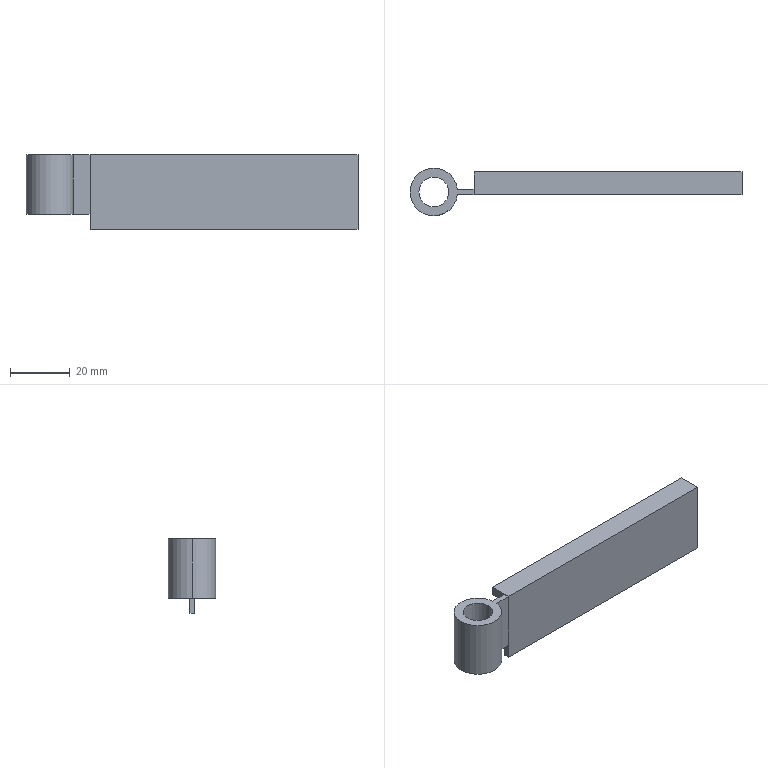Part | SolidWorks | features ICE 3, Extrusion 1 | 2 solids | 17 faces | box 111.5 x 16 x 25 mm | volume 8047 mm3 | plane 13 | cylinder 4 | commonest cylinder face diameters 10 x2 16 x2
STEP:
#1=CARTESIAN_POINT('',(-5.,0.,10.));
#2=VERTEX_POINT('',#1);
#3=CARTESIAN_POINT('',(5.,0.,10.));
#4=VERTEX_POINT('',#3);
#5=CARTESIAN_POINT('',(0.,0.,10.));
#6=DIRECTION('',(0.,0.,1.));
#7=DIRECTION('',(1.,0.,0.));
#8=AXIS2_PLACEMENT_3D('',#5,#6,#7);
#9=CIRCLE('',#8,5.);
#10=EDGE_CURVE('',#2,#4,#9,.T.);
#11=ORIENTED_EDGE('',*,*,#10,.T.);
#12=CARTESIAN_POINT('',(5.,0.,-10.));
#13=VERTEX_POINT('',#12);
#14=CARTESIAN_POINT('',(5.,0.,10.));
#15=DIRECTION('',(0.,0.,-1.));
#16=VECTOR('',#15,1000.);
#17=LINE('',#14,#16);
#18=EDGE_CURVE('',#4,#13,#17,.T.);
#19=ORIENTED_EDGE('',*,*,#18,.T.);
#20=CARTESIAN_POINT('',(-5.,0.,-10.));
#21=VERTEX_POINT('',#20);
#22=CARTESIAN_POINT('',(0.,0.,-10.));
#23=DIRECTION('',(0.,0.,1.));
#24=DIRECTION('',(1.,0.,0.));
#25=AXIS2_PLACEMENT_3D('',#22,#23,#24);
#26=CIRCLE('',#25,5.);
#27=EDGE_CURVE('',#21,#13,#26,.T.);
#28=ORIENTED_EDGE('',*,*,#27,.F.);
#29=CARTESIAN_POINT('',(-5.,0.,10.));
#30=DIRECTION('',(0.,0.,-1.));
#31=VECTOR('',#30,1000.);
#32=LINE('',#29,#31);
#33=EDGE_CURVE('',#2,#21,#32,.T.);
#34=ORIENTED_EDGE('',*,*,#33,.F.);
#35=EDGE_LOOP('',(#11,#19,#28,#34));
#36=FACE_OUTER_BOUND('',#35,.T.);
#37=CARTESIAN_POINT('',(0.,0.,10.));
#38=DIRECTION('',(0.,0.,-1.));
#39=DIRECTION('',(-1.,0.,0.));
#40=AXIS2_PLACEMENT_3D('',#37,#38,#39);
#41=CYLINDRICAL_SURFACE('',#40,5.);
#42=ADVANCED_FACE('',(#36),#41,.F.);
#43=CARTESIAN_POINT('',(-8.,0.,10.));
#44=VERTEX_POINT('',#43);
#45=CARTESIAN_POINT('',(7.945,-0.9375,10.));
#46=VERTEX_POINT('',#45);
#47=CARTESIAN_POINT('',(0.,0.,10.));
#48=DIRECTION('',(0.,0.,1.));
#49=DIRECTION('',(1.,0.,0.));
#50=AXIS2_PLACEMENT_3D('',#47,#48,#49);
#51=CIRCLE('',#50,8.);
#52=EDGE_CURVE('',#44,#46,#51,.T.);
#53=ORIENTED_EDGE('',*,*,#52,.F.);
#54=CARTESIAN_POINT('',(-8.,0.,-10.));
#55=VERTEX_POINT('',#54);
#56=CARTESIAN_POINT('',(-8.,0.,10.));
#57=DIRECTION('',(0.,0.,-1.));
#58=VECTOR('',#57,1000.);
#59=LINE('',#56,#58);
#60=EDGE_CURVE('',#44,#55,#59,.T.);
#61=ORIENTED_EDGE('',*,*,#60,.T.);
#62=CARTESIAN_POINT('',(7.945,-0.9375,-10.));
#63=VERTEX_POINT('',#62);
#64=CARTESIAN_POINT('',(0.,0.,-10.));
#65=DIRECTION('',(0.,0.,1.));
#66=DIRECTION('',(1.,0.,0.));
#67=AXIS2_PLACEMENT_3D('',#64,#65,#66);
#68=CIRCLE('',#67,8.);
#69=EDGE_CURVE('',#55,#63,#68,.T.);
#70=ORIENTED_EDGE('',*,*,#69,.T.);
#71=CARTESIAN_POINT('',(7.945,-0.9375,10.));
#72=DIRECTION('',(0.,0.,-1.));
#73=VECTOR('',#72,1000.);
#74=LINE('',#71,#73);
#75=EDGE_CURVE('',#46,#63,#74,.T.);
#76=ORIENTED_EDGE('',*,*,#75,.F.);
#77=EDGE_LOOP('',(#53,#61,#70,#76));
#78=FACE_OUTER_BOUND('',#77,.T.);
#79=CARTESIAN_POINT('',(0.,0.,10.));
#80=DIRECTION('',(0.,0.,-1.));
#81=DIRECTION('',(-1.,0.,0.));
#82=AXIS2_PLACEMENT_3D('',#79,#80,#81);
#83=CYLINDRICAL_SURFACE('',#82,8.);
#84=ADVANCED_FACE('',(#78),#83,.T.);
#85=ORIENTED_EDGE('',*,*,#60,.F.);
#86=CARTESIAN_POINT('',(7.945,0.9375,10.));
#87=VERTEX_POINT('',#86);
#88=CARTESIAN_POINT('',(0.,0.,10.));
#89=DIRECTION('',(0.,0.,1.));
#90=DIRECTION('',(1.,0.,0.));
#91=AXIS2_PLACEMENT_3D('',#88,#89,#90);
#92=CIRCLE('',#91,8.);
#93=EDGE_CURVE('',#87,#44,#92,.T.);
#94=ORIENTED_EDGE('',*,*,#93,.F.);
#95=CARTESIAN_POINT('',(7.945,0.9375,-10.));
#96=VERTEX_POINT('',#95);
#97=CARTESIAN_POINT('',(7.945,0.9375,10.));
#98=DIRECTION('',(0.,0.,1.));
#99=VECTOR('',#98,1000.);
#100=LINE('',#97,#99);
#101=EDGE_CURVE('',#96,#87,#100,.T.);
#102=ORIENTED_EDGE('',*,*,#101,.F.);
#103=CARTESIAN_POINT('',(0.,0.,-10.));
#104=DIRECTION('',(0.,0.,1.));
#105=DIRECTION('',(1.,0.,0.));
#106=AXIS2_PLACEMENT_3D('',#103,#104,#105);
#107=CIRCLE('',#106,8.);
#108=EDGE_CURVE('',#96,#55,#107,.T.);
#109=ORIENTED_EDGE('',*,*,#108,.T.);
#110=EDGE_LOOP('',(#85,#94,#102,#109));
#111=FACE_OUTER_BOUND('',#110,.T.);
#112=CARTESIAN_POINT('',(0.,0.,10.));
#113=DIRECTION('',(0.,0.,-1.));
#114=DIRECTION('',(-1.,0.,0.));
#115=AXIS2_PLACEMENT_3D('',#112,#113,#114);
#116=CYLINDRICAL_SURFACE('',#115,8.);
#117=ADVANCED_FACE('',(#111),#116,.T.);
#118=CARTESIAN_POINT('',(13.5,0.9375,10.));
#119=VERTEX_POINT('',#118);
#120=CARTESIAN_POINT('',(5.5,0.9375,10.));
#121=DIRECTION('',(-1.,0.,0.));
#122=VECTOR('',#121,1000.);
#123=LINE('',#120,#122);
#124=EDGE_CURVE('',#119,#87,#123,.T.);
#125=ORIENTED_EDGE('',*,*,#124,.T.);
#126=ORIENTED_EDGE('',*,*,#93,.T.);
#127=ORIENTED_EDGE('',*,*,#52,.T.);
#128=CARTESIAN_POINT('',(13.5,-0.9375,10.));
#129=VERTEX_POINT('',#128);
#130=CARTESIAN_POINT('',(5.5,-0.9375,10.));
#131=DIRECTION('',(1.,0.,0.));
#132=VECTOR('',#131,1000.);
#133=LINE('',#130,#132);
#134=EDGE_CURVE('',#46,#129,#133,.T.);
#135=ORIENTED_EDGE('',*,*,#134,.T.);
#136=CARTESIAN_POINT('',(13.5,-0.9375,10.));
#137=DIRECTION('',(0.,1.,0.));
#138=VECTOR('',#137,1000.);
#139=LINE('',#136,#138);
#140=EDGE_CURVE('',#129,#119,#139,.T.);
#141=ORIENTED_EDGE('',*,*,#140,.T.);
#142=EDGE_LOOP('',(#125,#126,#127,#135,#141));
#143=FACE_OUTER_BOUND('',#142,.T.);
#144=ORIENTED_EDGE('',*,*,#10,.F.);
#145=CARTESIAN_POINT('',(0.,0.,10.));
#146=DIRECTION('',(0.,0.,1.));
#147=DIRECTION('',(1.,0.,0.));
#148=AXIS2_PLACEMENT_3D('',#145,#146,#147);
#149=CIRCLE('',#148,5.);
#150=EDGE_CURVE('',#4,#2,#149,.T.);
#151=ORIENTED_EDGE('',*,*,#150,.F.);
#152=EDGE_LOOP('',(#144,#151));
#153=FACE_BOUND('',#152,.T.);
#154=CARTESIAN_POINT('',(0.,0.,10.));
#155=DIRECTION('',(0.,0.,1.));
#156=DIRECTION('',(1.,0.,0.));
#157=AXIS2_PLACEMENT_3D('',#154,#155,#156);
#158=PLANE('',#157);
#159=ADVANCED_FACE('',(#143,#153),#158,.T.);
#160=ORIENTED_EDGE('',*,*,#108,.F.);
#161=CARTESIAN_POINT('',(13.5,0.9375,-10.));
#162=VERTEX_POINT('',#161);
#163=CARTESIAN_POINT('',(5.5,0.9375,-10.));
#164=DIRECTION('',(-1.,0.,0.));
#165=VECTOR('',#164,1000.);
#166=LINE('',#163,#165);
#167=EDGE_CURVE('',#162,#96,#166,.T.);
#168=ORIENTED_EDGE('',*,*,#167,.F.);
#169=CARTESIAN_POINT('',(13.5,-0.9375,-10.));
#170=VERTEX_POINT('',#169);
#171=CARTESIAN_POINT('',(13.5,-0.9375,-10.));
#172=DIRECTION('',(0.,1.,0.));
#173=VECTOR('',#172,1000.);
#174=LINE('',#171,#173);
#175=EDGE_CURVE('',#170,#162,#174,.T.);
#176=ORIENTED_EDGE('',*,*,#175,.F.);
#177=CARTESIAN_POINT('',(5.5,-0.9375,-10.));
#178=DIRECTION('',(1.,0.,0.));
#179=VECTOR('',#178,1000.);
#180=LINE('',#177,#179);
#181=EDGE_CURVE('',#63,#170,#180,.T.);
#182=ORIENTED_EDGE('',*,*,#181,.F.);
#183=ORIENTED_EDGE('',*,*,#69,.F.);
#184=EDGE_LOOP('',(#160,#168,#176,#182,#183));
#185=FACE_OUTER_BOUND('',#184,.T.);
#186=ORIENTED_EDGE('',*,*,#27,.T.);
#187=CARTESIAN_POINT('',(0.,0.,-10.));
#188=DIRECTION('',(0.,0.,1.));
#189=DIRECTION('',(1.,0.,0.));
#190=AXIS2_PLACEMENT_3D('',#187,#188,#189);
#191=CIRCLE('',#190,5.);
#192=EDGE_CURVE('',#13,#21,#191,.T.);
#193=ORIENTED_EDGE('',*,*,#192,.T.);
#194=EDGE_LOOP('',(#186,#193));
#195=FACE_BOUND('',#194,.T.);
#196=CARTESIAN_POINT('',(0.,0.,-10.));
#197=DIRECTION('',(0.,0.,1.));
#198=DIRECTION('',(1.,0.,0.));
#199=AXIS2_PLACEMENT_3D('',#196,#197,#198);
#200=PLANE('',#199);
#201=ADVANCED_FACE('',(#185,#195),#200,.F.);
#202=ORIENTED_EDGE('',*,*,#18,.F.);
#203=ORIENTED_EDGE('',*,*,#150,.T.);
#204=ORIENTED_EDGE('',*,*,#33,.T.);
#205=ORIENTED_EDGE('',*,*,#192,.F.);
#206=EDGE_LOOP('',(#202,#203,#204,#205));
#207=FACE_OUTER_BOUND('',#206,.T.);
#208=CARTESIAN_POINT('',(0.,0.,10.));
#209=DIRECTION('',(0.,0.,-1.));
#210=DIRECTION('',(-1.,0.,0.));
#211=AXIS2_PLACEMENT_3D('',#208,#209,#210);
#212=CYLINDRICAL_SURFACE('',#211,5.);
#213=ADVANCED_FACE('',(#207),#212,.F.);
#214=ORIENTED_EDGE('',*,*,#167,.T.);
#215=ORIENTED_EDGE('',*,*,#101,.T.);
#216=ORIENTED_EDGE('',*,*,#124,.F.);
#217=CARTESIAN_POINT('',(13.5,0.9375,10.));
#218=DIRECTION('',(0.,0.,-1.));
#219=VECTOR('',#218,1000.);
#220=LINE('',#217,#219);
#221=EDGE_CURVE('',#119,#162,#220,.T.);
#222=ORIENTED_EDGE('',*,*,#221,.T.);
#223=EDGE_LOOP('',(#214,#215,#216,#222));
#224=FACE_OUTER_BOUND('',#223,.T.);
#225=CARTESIAN_POINT('',(5.5,0.9375,10.));
#226=DIRECTION('',(0.,-1.,0.));
#227=DIRECTION('',(0.,0.,-1.));
#228=AXIS2_PLACEMENT_3D('',#225,#226,#227);
#229=PLANE('',#228);
#230=ADVANCED_FACE('',(#224),#229,.F.);
#231=ORIENTED_EDGE('',*,*,#134,.F.);
#232=ORIENTED_EDGE('',*,*,#75,.T.);
#233=ORIENTED_EDGE('',*,*,#181,.T.);
#234=CARTESIAN_POINT('',(13.5,-0.9375,10.));
#235=DIRECTION('',(0.,0.,-1.));
#236=VECTOR('',#235,1000.);
#237=LINE('',#234,#236);
#238=EDGE_CURVE('',#129,#170,#237,.T.);
#239=ORIENTED_EDGE('',*,*,#238,.F.);
#240=EDGE_LOOP('',(#231,#232,#233,#239));
#241=FACE_OUTER_BOUND('',#240,.T.);
#242=CARTESIAN_POINT('',(5.5,-0.9375,10.));
#243=DIRECTION('',(0.,1.,0.));
#244=DIRECTION('',(0.,0.,1.));
#245=AXIS2_PLACEMENT_3D('',#242,#243,#244);
#246=PLANE('',#245);
#247=ADVANCED_FACE('',(#241),#246,.F.);
#248=ORIENTED_EDGE('',*,*,#175,.T.);
#249=ORIENTED_EDGE('',*,*,#221,.F.);
#250=ORIENTED_EDGE('',*,*,#140,.F.);
#251=ORIENTED_EDGE('',*,*,#238,.T.);
#252=EDGE_LOOP('',(#248,#249,#250,#251));
#253=FACE_OUTER_BOUND('',#252,.T.);
#254=CARTESIAN_POINT('',(13.5,-0.9375,10.));
#255=DIRECTION('',(-1.,0.,0.));
#256=DIRECTION('',(0.,0.,1.));
#257=AXIS2_PLACEMENT_3D('',#254,#255,#256);
#258=PLANE('',#257);
#259=ADVANCED_FACE('',(#253),#258,.F.);
#260=CLOSED_SHELL('',(#42,#84,#117,#159,#201,#213,#230,#247,#259));
#261=MANIFOLD_SOLID_BREP('',#260);
#262=CARTESIAN_POINT('',(13.5,0.7377,-15.));
#263=VERTEX_POINT('',#262);
#264=CARTESIAN_POINT('',(13.5,-0.9375,-15.));
#265=VERTEX_POINT('',#264);
#266=CARTESIAN_POINT('',(13.5,-0.9375,-15.));
#267=DIRECTION('',(0.,-1.,0.));
#268=VECTOR('',#267,1000.);
#269=LINE('',#266,#268);
#270=EDGE_CURVE('',#263,#265,#269,.T.);
#271=ORIENTED_EDGE('',*,*,#270,.F.);
#272=CARTESIAN_POINT('',(103.5,0.7377,-15.));
#273=VERTEX_POINT('',#272);
#274=CARTESIAN_POINT('',(13.5,0.7377,-15.));
#275=DIRECTION('',(-1.,0.,0.));
#276=VECTOR('',#275,1000.);
#277=LINE('',#274,#276);
#278=EDGE_CURVE('',#273,#263,#277,.T.);
#279=ORIENTED_EDGE('',*,*,#278,.F.);
#280=CARTESIAN_POINT('',(103.5,-0.9375,-15.));
#281=VERTEX_POINT('',#280);
#282=CARTESIAN_POINT('',(103.5,-0.9375,-15.));
#283=DIRECTION('',(0.,1.,0.));
#284=VECTOR('',#283,1000.);
#285=LINE('',#282,#284);
#286=EDGE_CURVE('',#281,#273,#285,.T.);
#287=ORIENTED_EDGE('',*,*,#286,.F.);
#288=CARTESIAN_POINT('',(13.5,-0.9375,-15.));
#289=DIRECTION('',(1.,0.,0.));
#290=VECTOR('',#289,1000.);
#291=LINE('',#288,#290);
#292=EDGE_CURVE('',#265,#281,#291,.T.);
#293=ORIENTED_EDGE('',*,*,#292,.F.);
#294=EDGE_LOOP('',(#271,#279,#287,#293));
#295=FACE_OUTER_BOUND('',#294,.T.);
#296=CARTESIAN_POINT('',(0.,0.,-15.));
#297=DIRECTION('',(0.,0.,-1.));
#298=DIRECTION('',(-1.,0.,0.));
#299=AXIS2_PLACEMENT_3D('',#296,#297,#298);
#300=PLANE('',#299);
#301=ADVANCED_FACE('',(#295),#300,.T.);
#302=CARTESIAN_POINT('',(13.5,0.7377,7.));
#303=VERTEX_POINT('',#302);
#304=CARTESIAN_POINT('',(13.5,6.738,7.));
#305=VERTEX_POINT('',#304);
#306=CARTESIAN_POINT('',(13.5,0.7377,7.));
#307=DIRECTION('',(0.,1.,0.));
#308=VECTOR('',#307,1000.);
#309=LINE('',#306,#308);
#310=EDGE_CURVE('',#303,#305,#309,.T.);
#311=ORIENTED_EDGE('',*,*,#310,.F.);
#312=CARTESIAN_POINT('',(13.5,0.7377,-15.));
#313=DIRECTION('',(0.,0.,1.));
#314=VECTOR('',#313,1000.);
#315=LINE('',#312,#314);
#316=EDGE_CURVE('',#263,#303,#315,.T.);
#317=ORIENTED_EDGE('',*,*,#316,.F.);
#318=ORIENTED_EDGE('',*,*,#270,.T.);
#319=CARTESIAN_POINT('',(13.5,-0.9375,10.));
#320=VERTEX_POINT('',#319);
#321=CARTESIAN_POINT('',(13.5,-0.9375,-15.));
#322=DIRECTION('',(0.,0.,1.));
#323=VECTOR('',#322,1000.);
#324=LINE('',#321,#323);
#325=EDGE_CURVE('',#265,#320,#324,.T.);
#326=ORIENTED_EDGE('',*,*,#325,.T.);
#327=CARTESIAN_POINT('',(13.5,6.738,10.));
#328=VERTEX_POINT('',#327);
#329=CARTESIAN_POINT('',(13.5,-0.9375,10.));
#330=DIRECTION('',(0.,-1.,0.));
#331=VECTOR('',#330,1000.);
#332=LINE('',#329,#331);
#333=EDGE_CURVE('',#328,#320,#332,.T.);
#334=ORIENTED_EDGE('',*,*,#333,.F.);
#335=CARTESIAN_POINT('',(13.5,6.738,-15.));
#336=DIRECTION('',(0.,0.,1.));
#337=VECTOR('',#336,1000.);
#338=LINE('',#335,#337);
#339=EDGE_CURVE('',#305,#328,#338,.T.);
#340=ORIENTED_EDGE('',*,*,#339,.F.);
#341=EDGE_LOOP('',(#311,#317,#318,#326,#334,#340));
#342=FACE_OUTER_BOUND('',#341,.T.);
#343=CARTESIAN_POINT('',(13.5,-0.9375,-15.));
#344=DIRECTION('',(-1.,0.,0.));
#345=DIRECTION('',(0.,0.,1.));
#346=AXIS2_PLACEMENT_3D('',#343,#344,#345);
#347=PLANE('',#346);
#348=ADVANCED_FACE('',(#342),#347,.T.);
#349=CARTESIAN_POINT('',(103.5,6.738,7.));
#350=VERTEX_POINT('',#349);
#351=CARTESIAN_POINT('',(13.5,6.738,7.));
#352=DIRECTION('',(1.,0.,0.));
#353=VECTOR('',#352,1000.);
#354=LINE('',#351,#353);
#355=EDGE_CURVE('',#305,#350,#354,.T.);
#356=ORIENTED_EDGE('',*,*,#355,.F.);
#357=ORIENTED_EDGE('',*,*,#339,.T.);
#358=CARTESIAN_POINT('',(103.5,6.738,10.));
#359=VERTEX_POINT('',#358);
#360=CARTESIAN_POINT('',(13.5,6.738,10.));
#361=DIRECTION('',(-1.,0.,0.));
#362=VECTOR('',#361,1000.);
#363=LINE('',#360,#362);
#364=EDGE_CURVE('',#359,#328,#363,.T.);
#365=ORIENTED_EDGE('',*,*,#364,.F.);
#366=CARTESIAN_POINT('',(103.5,6.738,-15.));
#367=DIRECTION('',(0.,0.,1.));
#368=VECTOR('',#367,1000.);
#369=LINE('',#366,#368);
#370=EDGE_CURVE('',#350,#359,#369,.T.);
#371=ORIENTED_EDGE('',*,*,#370,.F.);
#372=EDGE_LOOP('',(#356,#357,#365,#371));
#373=FACE_OUTER_BOUND('',#372,.T.);
#374=CARTESIAN_POINT('',(13.5,6.738,-15.));
#375=DIRECTION('',(0.,1.,0.));
#376=DIRECTION('',(0.,0.,1.));
#377=AXIS2_PLACEMENT_3D('',#374,#375,#376);
#378=PLANE('',#377);
#379=ADVANCED_FACE('',(#373),#378,.T.);
#380=CARTESIAN_POINT('',(103.5,0.7377,7.));
#381=VERTEX_POINT('',#380);
#382=CARTESIAN_POINT('',(103.5,0.7377,7.));
#383=DIRECTION('',(0.,1.,0.));
#384=VECTOR('',#383,1000.);
#385=LINE('',#382,#384);
#386=EDGE_CURVE('',#381,#350,#385,.T.);
#387=ORIENTED_EDGE('',*,*,#386,.T.);
#388=ORIENTED_EDGE('',*,*,#370,.T.);
#389=CARTESIAN_POINT('',(103.5,-0.9375,10.));
#390=VERTEX_POINT('',#389);
#391=CARTESIAN_POINT('',(103.5,-0.9375,10.));
#392=DIRECTION('',(0.,1.,0.));
#393=VECTOR('',#392,1000.);
#394=LINE('',#391,#393);
#395=EDGE_CURVE('',#390,#359,#394,.T.);
#396=ORIENTED_EDGE('',*,*,#395,.F.);
#397=CARTESIAN_POINT('',(103.5,-0.9375,-15.));
#398=DIRECTION('',(0.,0.,1.));
#399=VECTOR('',#398,1000.);
#400=LINE('',#397,#399);
#401=EDGE_CURVE('',#281,#390,#400,.T.);
#402=ORIENTED_EDGE('',*,*,#401,.F.);
#403=ORIENTED_EDGE('',*,*,#286,.T.);
#404=CARTESIAN_POINT('',(103.5,0.7377,-15.));
#405=DIRECTION('',(0.,0.,-1.));
#406=VECTOR('',#405,1000.);
#407=LINE('',#404,#406);
#408=EDGE_CURVE('',#381,#273,#407,.T.);
#409=ORIENTED_EDGE('',*,*,#408,.F.);
#410=EDGE_LOOP('',(#387,#388,#396,#402,#403,#409));
#411=FACE_OUTER_BOUND('',#410,.T.);
#412=CARTESIAN_POINT('',(103.5,-0.9375,-15.));
#413=DIRECTION('',(1.,0.,0.));
#414=DIRECTION('',(0.,0.,-1.));
#415=AXIS2_PLACEMENT_3D('',#412,#413,#414);
#416=PLANE('',#415);
#417=ADVANCED_FACE('',(#411),#416,.T.);
#418=CARTESIAN_POINT('',(13.5,-0.9375,10.));
#419=DIRECTION('',(1.,0.,0.));
#420=VECTOR('',#419,1000.);
#421=LINE('',#418,#420);
#422=EDGE_CURVE('',#320,#390,#421,.T.);
#423=ORIENTED_EDGE('',*,*,#422,.F.);
#424=ORIENTED_EDGE('',*,*,#325,.F.);
#425=ORIENTED_EDGE('',*,*,#292,.T.);
#426=ORIENTED_EDGE('',*,*,#401,.T.);
#427=EDGE_LOOP('',(#423,#424,#425,#426));
#428=FACE_OUTER_BOUND('',#427,.T.);
#429=CARTESIAN_POINT('',(13.5,-0.9375,-15.));
#430=DIRECTION('',(0.,-1.,0.));
#431=DIRECTION('',(0.,0.,-1.));
#432=AXIS2_PLACEMENT_3D('',#429,#430,#431);
#433=PLANE('',#432);
#434=ADVANCED_FACE('',(#428),#433,.T.);
#435=ORIENTED_EDGE('',*,*,#333,.T.);
#436=ORIENTED_EDGE('',*,*,#422,.T.);
#437=ORIENTED_EDGE('',*,*,#395,.T.);
#438=ORIENTED_EDGE('',*,*,#364,.T.);
#439=EDGE_LOOP('',(#435,#436,#437,#438));
#440=FACE_OUTER_BOUND('',#439,.T.);
#441=CARTESIAN_POINT('',(0.,0.,10.));
#442=DIRECTION('',(0.,0.,-1.));
#443=DIRECTION('',(-1.,0.,0.));
#444=AXIS2_PLACEMENT_3D('',#441,#442,#443);
#445=PLANE('',#444);
#446=ADVANCED_FACE('',(#440),#445,.F.);
#447=ORIENTED_EDGE('',*,*,#355,.T.);
#448=ORIENTED_EDGE('',*,*,#386,.F.);
#449=CARTESIAN_POINT('',(13.5,0.7377,7.));
#450=DIRECTION('',(1.,0.,0.));
#451=VECTOR('',#450,1000.);
#452=LINE('',#449,#451);
#453=EDGE_CURVE('',#303,#381,#452,.T.);
#454=ORIENTED_EDGE('',*,*,#453,.F.);
#455=ORIENTED_EDGE('',*,*,#310,.T.);
#456=EDGE_LOOP('',(#447,#448,#454,#455));
#457=FACE_OUTER_BOUND('',#456,.T.);
#458=CARTESIAN_POINT('',(13.5,0.7377,7.));
#459=DIRECTION('',(0.,0.,1.));
#460=DIRECTION('',(1.,0.,0.));
#461=AXIS2_PLACEMENT_3D('',#458,#459,#460);
#462=PLANE('',#461);
#463=ADVANCED_FACE('',(#457),#462,.F.);
#464=ORIENTED_EDGE('',*,*,#316,.T.);
#465=ORIENTED_EDGE('',*,*,#453,.T.);
#466=ORIENTED_EDGE('',*,*,#408,.T.);
#467=ORIENTED_EDGE('',*,*,#278,.T.);
#468=EDGE_LOOP('',(#464,#465,#466,#467));
#469=FACE_OUTER_BOUND('',#468,.T.);
#470=CARTESIAN_POINT('',(0.,0.7377,0.));
#471=DIRECTION('',(0.,1.,0.));
#472=DIRECTION('',(0.,0.,1.));
#473=AXIS2_PLACEMENT_3D('',#470,#471,#472);
#474=PLANE('',#473);
#475=ADVANCED_FACE('',(#469),#474,.T.);
#476=CLOSED_SHELL('',(#301,#348,#379,#417,#434,#446,#463,#475));
#477=MANIFOLD_SOLID_BREP('',#476);
#478=CARTESIAN_POINT('',(0.,0.,0.));
#479=DIRECTION('',(0.,0.,1.));
#480=DIRECTION('',(1.,0.,0.));
#481=AXIS2_PLACEMENT_3D('',#478,#479,#480);
#482=(LENGTH_UNIT()NAMED_UNIT(*)SI_UNIT(.MILLI.,.METRE.));
#483=UNCERTAINTY_MEASURE_WITH_UNIT(LENGTH_MEASURE(0.00001),#482,'','');
#484=(NAMED_UNIT(*)PLANE_ANGLE_UNIT()SI_UNIT($,.RADIAN.));
#485=(NAMED_UNIT(*)SI_UNIT($,.STERADIAN.)SOLID_ANGLE_UNIT());
#486=(GEOMETRIC_REPRESENTATION_CONTEXT(3)GLOBAL_UNCERTAINTY_ASSIGNED_CONTEXT((#483))GLOBAL_UNIT_ASSIGNED_CONTEXT((#482,#484,#485))REPRESENTATION_CONTEXT('',''));
#487=ADVANCED_BREP_SHAPE_REPRESENTATION('',(#261,#477,#481),#486);